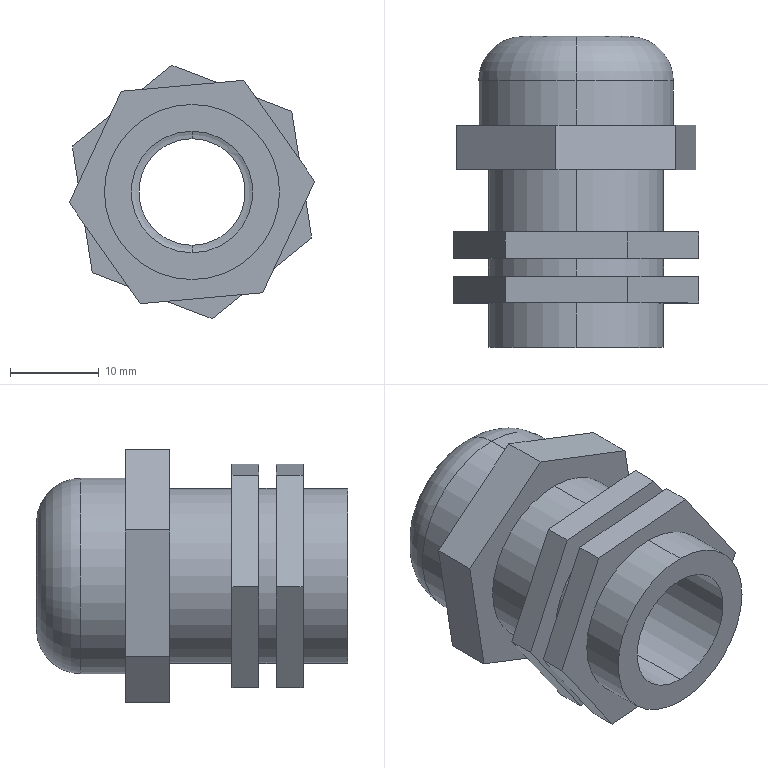Part | SolidWorks | features ICE 5, Extrusion 1, Fillet 1, Shell 1 | 1 solid | 44 faces | box 27.604 x 35 x 28.514 mm | volume 7936 mm3 | plane 26 | cylinder 14 | torus 4 | commonest cylinder face diameters 19.7 x6 12 x2 13.7 x2 16 x2 22 x2
STEP:
#1=CARTESIAN_POINT('',(0.,23.,-6.85));
#2=VERTEX_POINT('',#1);
#3=CARTESIAN_POINT('',(0.,23.,6.85));
#4=VERTEX_POINT('',#3);
#5=CARTESIAN_POINT('',(0.,23.,0.));
#6=DIRECTION('',(0.,1.,0.));
#7=DIRECTION('',(0.,0.,1.));
#8=AXIS2_PLACEMENT_3D('',#5,#6,#7);
#9=CIRCLE('',#8,6.85);
#10=EDGE_CURVE('',#2,#4,#9,.T.);
#11=ORIENTED_EDGE('',*,*,#10,.T.);
#12=CARTESIAN_POINT('',(0.,0.,6.85));
#13=VERTEX_POINT('',#12);
#14=CARTESIAN_POINT('',(0.,20.,6.85));
#15=DIRECTION('',(0.,-1.,0.));
#16=VECTOR('',#15,1000.);
#17=LINE('',#14,#16);
#18=EDGE_CURVE('',#4,#13,#17,.T.);
#19=ORIENTED_EDGE('',*,*,#18,.T.);
#20=CARTESIAN_POINT('',(0.,0.,-6.85));
#21=VERTEX_POINT('',#20);
#22=CARTESIAN_POINT('',(0.,0.,0.));
#23=DIRECTION('',(0.,1.,0.));
#24=DIRECTION('',(0.,0.,1.));
#25=AXIS2_PLACEMENT_3D('',#22,#23,#24);
#26=CIRCLE('',#25,6.85);
#27=EDGE_CURVE('',#21,#13,#26,.T.);
#28=ORIENTED_EDGE('',*,*,#27,.F.);
#29=CARTESIAN_POINT('',(0.,20.,-6.85));
#30=DIRECTION('',(0.,-1.,0.));
#31=VECTOR('',#30,1000.);
#32=LINE('',#29,#31);
#33=EDGE_CURVE('',#2,#21,#32,.T.);
#34=ORIENTED_EDGE('',*,*,#33,.F.);
#35=EDGE_LOOP('',(#11,#19,#28,#34));
#36=FACE_OUTER_BOUND('',#35,.T.);
#37=CARTESIAN_POINT('',(0.,20.,0.));
#38=DIRECTION('',(0.,-1.,0.));
#39=DIRECTION('',(0.,0.,-1.));
#40=AXIS2_PLACEMENT_3D('',#37,#38,#39);
#41=CYLINDRICAL_SURFACE('',#40,6.85);
#42=ADVANCED_FACE('',(#36),#41,.F.);
#43=CARTESIAN_POINT('',(0.,5.,-9.85));
#44=VERTEX_POINT('',#43);
#45=CARTESIAN_POINT('',(0.,5.,9.85));
#46=VERTEX_POINT('',#45);
#47=CARTESIAN_POINT('',(0.,5.,0.));
#48=DIRECTION('',(0.,-1.,0.));
#49=DIRECTION('',(0.,0.,-1.));
#50=AXIS2_PLACEMENT_3D('',#47,#48,#49);
#51=CIRCLE('',#50,9.85);
#52=EDGE_CURVE('',#44,#46,#51,.T.);
#53=ORIENTED_EDGE('',*,*,#52,.T.);
#54=CARTESIAN_POINT('',(0.,0.,9.85));
#55=VERTEX_POINT('',#54);
#56=CARTESIAN_POINT('',(0.,20.,9.85));
#57=DIRECTION('',(0.,-1.,0.));
#58=VECTOR('',#57,1000.);
#59=LINE('',#56,#58);
#60=EDGE_CURVE('',#46,#55,#59,.T.);
#61=ORIENTED_EDGE('',*,*,#60,.T.);
#62=CARTESIAN_POINT('',(0.,0.,-9.85));
#63=VERTEX_POINT('',#62);
#64=CARTESIAN_POINT('',(0.,0.,0.));
#65=DIRECTION('',(0.,1.,0.));
#66=DIRECTION('',(0.,0.,1.));
#67=AXIS2_PLACEMENT_3D('',#64,#65,#66);
#68=CIRCLE('',#67,9.85);
#69=EDGE_CURVE('',#55,#63,#68,.T.);
#70=ORIENTED_EDGE('',*,*,#69,.T.);
#71=CARTESIAN_POINT('',(0.,20.,-9.85));
#72=DIRECTION('',(0.,-1.,0.));
#73=VECTOR('',#72,1000.);
#74=LINE('',#71,#73);
#75=EDGE_CURVE('',#44,#63,#74,.T.);
#76=ORIENTED_EDGE('',*,*,#75,.F.);
#77=EDGE_LOOP('',(#53,#61,#70,#76));
#78=FACE_OUTER_BOUND('',#77,.T.);
#79=CARTESIAN_POINT('',(0.,20.,0.));
#80=DIRECTION('',(0.,-1.,0.));
#81=DIRECTION('',(0.,0.,-1.));
#82=AXIS2_PLACEMENT_3D('',#79,#80,#81);
#83=CYLINDRICAL_SURFACE('',#82,9.85);
#84=ADVANCED_FACE('',(#78),#83,.T.);
#85=CARTESIAN_POINT('',(0.,30.,8.));
#86=VERTEX_POINT('',#85);
#87=CARTESIAN_POINT('',(0.,30.,-8.));
#88=VERTEX_POINT('',#87);
#89=CARTESIAN_POINT('',(0.,30.,0.));
#90=DIRECTION('',(0.,-1.,0.));
#91=DIRECTION('',(0.,0.,-1.));
#92=AXIS2_PLACEMENT_3D('',#89,#90,#91);
#93=CIRCLE('',#92,8.);
#94=EDGE_CURVE('',#86,#88,#93,.T.);
#95=ORIENTED_EDGE('',*,*,#94,.T.);
#96=CARTESIAN_POINT('',(0.,32.,-6.));
#97=VERTEX_POINT('',#96);
#98=CARTESIAN_POINT('',(0.,30.,-6.));
#99=DIRECTION('',(1.,0.,0.));
#100=DIRECTION('',(0.,0.,-1.));
#101=AXIS2_PLACEMENT_3D('',#98,#99,#100);
#102=CIRCLE('',#101,2.);
#103=EDGE_CURVE('',#88,#97,#102,.T.);
#104=ORIENTED_EDGE('',*,*,#103,.T.);
#105=CARTESIAN_POINT('',(0.,32.,6.));
#106=VERTEX_POINT('',#105);
#107=CARTESIAN_POINT('',(0.,32.,0.));
#108=DIRECTION('',(0.,1.,0.));
#109=DIRECTION('',(0.,0.,-1.));
#110=AXIS2_PLACEMENT_3D('',#107,#108,#109);
#111=CIRCLE('',#110,6.);
#112=EDGE_CURVE('',#97,#106,#111,.T.);
#113=ORIENTED_EDGE('',*,*,#112,.T.);
#114=CARTESIAN_POINT('',(0.,30.,6.));
#115=DIRECTION('',(-1.,0.,0.));
#116=DIRECTION('',(0.,0.,1.));
#117=AXIS2_PLACEMENT_3D('',#114,#115,#116);
#118=CIRCLE('',#117,2.);
#119=EDGE_CURVE('',#86,#106,#118,.T.);
#120=ORIENTED_EDGE('',*,*,#119,.F.);
#121=EDGE_LOOP('',(#95,#104,#113,#120));
#122=FACE_OUTER_BOUND('',#121,.T.);
#123=CARTESIAN_POINT('',(0.,30.,0.));
#124=DIRECTION('',(0.,1.,0.));
#125=DIRECTION('',(0.,0.,1.));
#126=AXIS2_PLACEMENT_3D('',#123,#124,#125);
#127=TOROIDAL_SURFACE('',#126,6.,2.);
#128=ADVANCED_FACE('',(#122),#127,.F.);
#129=ORIENTED_EDGE('',*,*,#94,.F.);
#130=CARTESIAN_POINT('',(0.,23.,8.));
#131=VERTEX_POINT('',#130);
#132=CARTESIAN_POINT('',(0.,35.,8.));
#133=DIRECTION('',(0.,-1.,0.));
#134=VECTOR('',#133,1000.);
#135=LINE('',#132,#134);
#136=EDGE_CURVE('',#86,#131,#135,.T.);
#137=ORIENTED_EDGE('',*,*,#136,.T.);
#138=CARTESIAN_POINT('',(0.,23.,-8.));
#139=VERTEX_POINT('',#138);
#140=CARTESIAN_POINT('',(0.,23.,0.));
#141=DIRECTION('',(0.,-1.,0.));
#142=DIRECTION('',(0.,0.,1.));
#143=AXIS2_PLACEMENT_3D('',#140,#141,#142);
#144=CIRCLE('',#143,8.);
#145=EDGE_CURVE('',#131,#139,#144,.T.);
#146=ORIENTED_EDGE('',*,*,#145,.T.);
#147=CARTESIAN_POINT('',(0.,35.,-8.));
#148=DIRECTION('',(0.,-1.,0.));
#149=VECTOR('',#148,1000.);
#150=LINE('',#147,#149);
#151=EDGE_CURVE('',#88,#139,#150,.T.);
#152=ORIENTED_EDGE('',*,*,#151,.F.);
#153=EDGE_LOOP('',(#129,#137,#146,#152));
#154=FACE_OUTER_BOUND('',#153,.T.);
#155=CARTESIAN_POINT('',(0.,35.,0.));
#156=DIRECTION('',(0.,-1.,0.));
#157=DIRECTION('',(0.,0.,-1.));
#158=AXIS2_PLACEMENT_3D('',#155,#156,#157);
#159=CYLINDRICAL_SURFACE('',#158,8.);
#160=ADVANCED_FACE('',(#154),#159,.F.);
#161=ORIENTED_EDGE('',*,*,#112,.F.);
#162=CARTESIAN_POINT('',(0.,35.,-6.));
#163=VERTEX_POINT('',#162);
#164=CARTESIAN_POINT('',(0.,35.,-6.));
#165=DIRECTION('',(0.,1.,0.));
#166=VECTOR('',#165,1000.);
#167=LINE('',#164,#166);
#168=EDGE_CURVE('',#97,#163,#167,.T.);
#169=ORIENTED_EDGE('',*,*,#168,.T.);
#170=CARTESIAN_POINT('',(0.,35.,6.));
#171=VERTEX_POINT('',#170);
#172=CARTESIAN_POINT('',(0.,35.,0.));
#173=DIRECTION('',(0.,1.,0.));
#174=DIRECTION('',(0.,0.,1.));
#175=AXIS2_PLACEMENT_3D('',#172,#173,#174);
#176=CIRCLE('',#175,6.);
#177=EDGE_CURVE('',#163,#171,#176,.T.);
#178=ORIENTED_EDGE('',*,*,#177,.T.);
#179=CARTESIAN_POINT('',(0.,35.,6.));
#180=DIRECTION('',(0.,1.,0.));
#181=VECTOR('',#180,1000.);
#182=LINE('',#179,#181);
#183=EDGE_CURVE('',#106,#171,#182,.T.);
#184=ORIENTED_EDGE('',*,*,#183,.F.);
#185=EDGE_LOOP('',(#161,#169,#178,#184));
#186=FACE_OUTER_BOUND('',#185,.T.);
#187=CARTESIAN_POINT('',(0.,35.,0.));
#188=DIRECTION('',(0.,1.,0.));
#189=DIRECTION('',(0.,0.,1.));
#190=AXIS2_PLACEMENT_3D('',#187,#188,#189);
#191=CYLINDRICAL_SURFACE('',#190,6.);
#192=ADVANCED_FACE('',(#186),#191,.F.);
#193=CARTESIAN_POINT('',(0.,30.,-11.));
#194=VERTEX_POINT('',#193);
#195=CARTESIAN_POINT('',(0.,30.,11.));
#196=VERTEX_POINT('',#195);
#197=CARTESIAN_POINT('',(0.,30.,0.));
#198=DIRECTION('',(0.,-1.,0.));
#199=DIRECTION('',(0.,0.,1.));
#200=AXIS2_PLACEMENT_3D('',#197,#198,#199);
#201=CIRCLE('',#200,11.);
#202=EDGE_CURVE('',#194,#196,#201,.T.);
#203=ORIENTED_EDGE('',*,*,#202,.F.);
#204=CARTESIAN_POINT('',(0.,30.,-6.));
#205=DIRECTION('',(1.,0.,0.));
#206=DIRECTION('',(0.,0.,-1.));
#207=AXIS2_PLACEMENT_3D('',#204,#205,#206);
#208=CIRCLE('',#207,5.);
#209=EDGE_CURVE('',#194,#163,#208,.T.);
#210=ORIENTED_EDGE('',*,*,#209,.T.);
#211=CARTESIAN_POINT('',(0.,35.,0.));
#212=DIRECTION('',(0.,1.,0.));
#213=DIRECTION('',(0.,0.,1.));
#214=AXIS2_PLACEMENT_3D('',#211,#212,#213);
#215=CIRCLE('',#214,6.);
#216=EDGE_CURVE('',#171,#163,#215,.T.);
#217=ORIENTED_EDGE('',*,*,#216,.F.);
#218=CARTESIAN_POINT('',(0.,30.,6.));
#219=DIRECTION('',(-1.,0.,0.));
#220=DIRECTION('',(0.,0.,1.));
#221=AXIS2_PLACEMENT_3D('',#218,#219,#220);
#222=CIRCLE('',#221,5.);
#223=EDGE_CURVE('',#196,#171,#222,.T.);
#224=ORIENTED_EDGE('',*,*,#223,.F.);
#225=EDGE_LOOP('',(#203,#210,#217,#224));
#226=FACE_OUTER_BOUND('',#225,.T.);
#227=CARTESIAN_POINT('',(0.,30.,0.));
#228=DIRECTION('',(0.,1.,0.));
#229=DIRECTION('',(0.,0.,1.));
#230=AXIS2_PLACEMENT_3D('',#227,#228,#229);
#231=TOROIDAL_SURFACE('',#230,6.,5.);
#232=ADVANCED_FACE('',(#226),#231,.T.);
#233=ORIENTED_EDGE('',*,*,#202,.T.);
#234=CARTESIAN_POINT('',(0.,25.,11.));
#235=VERTEX_POINT('',#234);
#236=CARTESIAN_POINT('',(0.,35.,11.));
#237=DIRECTION('',(0.,-1.,0.));
#238=VECTOR('',#237,1000.);
#239=LINE('',#236,#238);
#240=EDGE_CURVE('',#196,#235,#239,.T.);
#241=ORIENTED_EDGE('',*,*,#240,.T.);
#242=CARTESIAN_POINT('',(0.,25.,-11.));
#243=VERTEX_POINT('',#242);
#244=CARTESIAN_POINT('',(0.,25.,0.));
#245=DIRECTION('',(0.,1.,0.));
#246=DIRECTION('',(0.,0.,1.));
#247=AXIS2_PLACEMENT_3D('',#244,#245,#246);
#248=CIRCLE('',#247,11.);
#249=EDGE_CURVE('',#235,#243,#248,.T.);
#250=ORIENTED_EDGE('',*,*,#249,.T.);
#251=CARTESIAN_POINT('',(0.,35.,-11.));
#252=DIRECTION('',(0.,-1.,0.));
#253=VECTOR('',#252,1000.);
#254=LINE('',#251,#253);
#255=EDGE_CURVE('',#194,#243,#254,.T.);
#256=ORIENTED_EDGE('',*,*,#255,.F.);
#257=EDGE_LOOP('',(#233,#241,#250,#256));
#258=FACE_OUTER_BOUND('',#257,.T.);
#259=CARTESIAN_POINT('',(0.,35.,0.));
#260=DIRECTION('',(0.,-1.,0.));
#261=DIRECTION('',(0.,0.,-1.));
#262=AXIS2_PLACEMENT_3D('',#259,#260,#261);
#263=CYLINDRICAL_SURFACE('',#262,11.);
#264=ADVANCED_FACE('',(#258),#263,.T.);
#265=CARTESIAN_POINT('',(0.,20.,9.85));
#266=VERTEX_POINT('',#265);
#267=CARTESIAN_POINT('',(0.,20.,-9.85));
#268=VERTEX_POINT('',#267);
#269=CARTESIAN_POINT('',(0.,20.,0.));
#270=DIRECTION('',(0.,1.,0.));
#271=DIRECTION('',(0.,0.,1.));
#272=AXIS2_PLACEMENT_3D('',#269,#270,#271);
#273=CIRCLE('',#272,9.85);
#274=EDGE_CURVE('',#266,#268,#273,.T.);
#275=ORIENTED_EDGE('',*,*,#274,.F.);
#276=CARTESIAN_POINT('',(0.,13.,9.85));
#277=VERTEX_POINT('',#276);
#278=CARTESIAN_POINT('',(0.,20.,9.85));
#279=DIRECTION('',(0.,-1.,0.));
#280=VECTOR('',#279,1000.);
#281=LINE('',#278,#280);
#282=EDGE_CURVE('',#266,#277,#281,.T.);
#283=ORIENTED_EDGE('',*,*,#282,.T.);
#284=CARTESIAN_POINT('',(0.,13.,-9.85));
#285=VERTEX_POINT('',#284);
#286=CARTESIAN_POINT('',(0.,13.,0.));
#287=DIRECTION('',(0.,-1.,0.));
#288=DIRECTION('',(0.,0.,-1.));
#289=AXIS2_PLACEMENT_3D('',#286,#287,#288);
#290=CIRCLE('',#289,9.85);
#291=EDGE_CURVE('',#285,#277,#290,.T.);
#292=ORIENTED_EDGE('',*,*,#291,.F.);
#293=CARTESIAN_POINT('',(0.,20.,-9.85));
#294=DIRECTION('',(0.,-1.,0.));
#295=VECTOR('',#294,1000.);
#296=LINE('',#293,#295);
#297=EDGE_CURVE('',#268,#285,#296,.T.);
#298=ORIENTED_EDGE('',*,*,#297,.F.);
#299=EDGE_LOOP('',(#275,#283,#292,#298));
#300=FACE_OUTER_BOUND('',#299,.T.);
#301=CARTESIAN_POINT('',(0.,20.,0.));
#302=DIRECTION('',(0.,-1.,0.));
#303=DIRECTION('',(0.,0.,-1.));
#304=AXIS2_PLACEMENT_3D('',#301,#302,#303);
#305=CYLINDRICAL_SURFACE('',#304,9.85);
#306=ADVANCED_FACE('',(#300),#305,.T.);
#307=CARTESIAN_POINT('',(0.,10.,-9.85));
#308=VERTEX_POINT('',#307);
#309=CARTESIAN_POINT('',(0.,10.,9.85));
#310=VERTEX_POINT('',#309);
#311=CARTESIAN_POINT('',(0.,10.,0.));
#312=DIRECTION('',(0.,-1.,0.));
#313=DIRECTION('',(0.,0.,-1.));
#314=AXIS2_PLACEMENT_3D('',#311,#312,#313);
#315=CIRCLE('',#314,9.85);
#316=EDGE_CURVE('',#308,#310,#315,.T.);
#317=ORIENTED_EDGE('',*,*,#316,.T.);
#318=CARTESIAN_POINT('',(0.,8.,9.85));
#319=VERTEX_POINT('',#318);
#320=CARTESIAN_POINT('',(0.,20.,9.85));
#321=DIRECTION('',(0.,-1.,0.));
#322=VECTOR('',#321,1000.);
#323=LINE('',#320,#322);
#324=EDGE_CURVE('',#310,#319,#323,.T.);
#325=ORIENTED_EDGE('',*,*,#324,.T.);
#326=CARTESIAN_POINT('',(0.,8.,-9.85));
#327=VERTEX_POINT('',#326);
#328=CARTESIAN_POINT('',(0.,8.,0.));
#329=DIRECTION('',(0.,-1.,0.));
#330=DIRECTION('',(0.,0.,-1.));
#331=AXIS2_PLACEMENT_3D('',#328,#329,#330);
#332=CIRCLE('',#331,9.85);
#333=EDGE_CURVE('',#327,#319,#332,.T.);
#334=ORIENTED_EDGE('',*,*,#333,.F.);
#335=CARTESIAN_POINT('',(0.,20.,-9.85));
#336=DIRECTION('',(0.,-1.,0.));
#337=VECTOR('',#336,1000.);
#338=LINE('',#335,#337);
#339=EDGE_CURVE('',#308,#327,#338,.T.);
#340=ORIENTED_EDGE('',*,*,#339,.F.);
#341=EDGE_LOOP('',(#317,#325,#334,#340));
#342=FACE_OUTER_BOUND('',#341,.T.);
#343=CARTESIAN_POINT('',(0.,20.,0.));
#344=DIRECTION('',(0.,-1.,0.));
#345=DIRECTION('',(0.,0.,-1.));
#346=AXIS2_PLACEMENT_3D('',#343,#344,#345);
#347=CYLINDRICAL_SURFACE('',#346,9.85);
#348=ADVANCED_FACE('',(#342),#347,.T.);
#349=ORIENTED_EDGE('',*,*,#324,.F.);
#350=CARTESIAN_POINT('',(0.,10.,0.));
#351=DIRECTION('',(0.,-1.,0.));
#352=DIRECTION('',(0.,0.,-1.));
#353=AXIS2_PLACEMENT_3D('',#350,#351,#352);
#354=CIRCLE('',#353,9.85);
#355=EDGE_CURVE('',#310,#308,#354,.T.);
#356=ORIENTED_EDGE('',*,*,#355,.T.);
#357=ORIENTED_EDGE('',*,*,#339,.T.);
#358=CARTESIAN_POINT('',(0.,8.,0.));
#359=DIRECTION('',(0.,-1.,0.));
#360=DIRECTION('',(0.,0.,-1.));
#361=AXIS2_PLACEMENT_3D('',#358,#359,#360);
#362=CIRCLE('',#361,9.85);
#363=EDGE_CURVE('',#319,#327,#362,.T.);
#364=ORIENTED_EDGE('',*,*,#363,.F.);
#365=EDGE_LOOP('',(#349,#356,#357,#364));
#366=FACE_OUTER_BOUND('',#365,.T.);
#367=CARTESIAN_POINT('',(0.,20.,0.));
#368=DIRECTION('',(0.,-1.,0.));
#369=DIRECTION('',(0.,0.,-1.));
#370=AXIS2_PLACEMENT_3D('',#367,#368,#369);
#371=CYLINDRICAL_SURFACE('',#370,9.85);
#372=ADVANCED_FACE('',(#366),#371,.T.);
#373=ORIENTED_EDGE('',*,*,#282,.F.);
#374=CARTESIAN_POINT('',(0.,20.,0.));
#375=DIRECTION('',(0.,1.,0.));
#376=DIRECTION('',(0.,0.,1.));
#377=AXIS2_PLACEMENT_3D('',#374,#375,#376);
#378=CIRCLE('',#377,9.85);
#379=EDGE_CURVE('',#268,#266,#378,.T.);
#380=ORIENTED_EDGE('',*,*,#379,.F.);
#381=ORIENTED_EDGE('',*,*,#297,.T.);
#382=CARTESIAN_POINT('',(0.,13.,0.));
#383=DIRECTION('',(0.,-1.,0.));
#384=DIRECTION('',(0.,0.,-1.));
#385=AXIS2_PLACEMENT_3D('',#382,#383,#384);
#386=CIRCLE('',#385,9.85);
#387=EDGE_CURVE('',#277,#285,#386,.T.);
#388=ORIENTED_EDGE('',*,*,#387,.F.);
#389=EDGE_LOOP('',(#373,#380,#381,#388));
#390=FACE_OUTER_BOUND('',#389,.T.);
#391=CARTESIAN_POINT('',(0.,20.,0.));
#392=DIRECTION('',(0.,-1.,0.));
#393=DIRECTION('',(0.,0.,-1.));
#394=AXIS2_PLACEMENT_3D('',#391,#392,#393);
#395=CYLINDRICAL_SURFACE('',#394,9.85);
#396=ADVANCED_FACE('',(#390),#395,.T.);
#397=CARTESIAN_POINT('',(13.473,20.,-5.178));
#398=VERTEX_POINT('',#397);
#399=CARTESIAN_POINT('',(2.253,20.,-14.257));
#400=VERTEX_POINT('',#399);
#401=CARTESIAN_POINT('',(13.473,20.,-5.178));
#402=DIRECTION('',(-0.7774,0.,-0.629));
#403=VECTOR('',#402,1000.);
#404=LINE('',#401,#403);
#405=EDGE_CURVE('',#398,#400,#404,.T.);
#406=ORIENTED_EDGE('',*,*,#405,.T.);
#407=CARTESIAN_POINT('',(2.253,25.,-14.257));
#408=VERTEX_POINT('',#407);
#409=CARTESIAN_POINT('',(2.253,25.,-14.257));
#410=DIRECTION('',(0.,-1.,0.));
#411=VECTOR('',#410,1000.);
#412=LINE('',#409,#411);
#413=EDGE_CURVE('',#408,#400,#412,.T.);
#414=ORIENTED_EDGE('',*,*,#413,.F.);
#415=CARTESIAN_POINT('',(13.473,25.,-5.178));
#416=VERTEX_POINT('',#415);
#417=CARTESIAN_POINT('',(13.473,25.,-5.178));
#418=DIRECTION('',(-0.7774,0.,-0.629));
#419=VECTOR('',#418,1000.);
#420=LINE('',#417,#419);
#421=EDGE_CURVE('',#416,#408,#420,.T.);
#422=ORIENTED_EDGE('',*,*,#421,.F.);
#423=CARTESIAN_POINT('',(13.473,25.,-5.178));
#424=DIRECTION('',(0.,-1.,0.));
#425=VECTOR('',#424,1000.);
#426=LINE('',#423,#425);
#427=EDGE_CURVE('',#416,#398,#426,.T.);
#428=ORIENTED_EDGE('',*,*,#427,.T.);
#429=EDGE_LOOP('',(#406,#414,#422,#428));
#430=FACE_OUTER_BOUND('',#429,.T.);
#431=CARTESIAN_POINT('',(13.473,25.,-5.178));
#432=DIRECTION('',(-0.629,0.,0.7774));
#433=DIRECTION('',(0.7774,0.,0.629));
#434=AXIS2_PLACEMENT_3D('',#431,#432,#433);
#435=PLANE('',#434);
#436=ADVANCED_FACE('',(#430),#435,.F.);
#437=CARTESIAN_POINT('',(-11.221,20.,-9.079));
#438=VERTEX_POINT('',#437);
#439=CARTESIAN_POINT('',(2.253,20.,-14.257));
#440=DIRECTION('',(-0.9334,0.,0.3587));
#441=VECTOR('',#440,1000.);
#442=LINE('',#439,#441);
#443=EDGE_CURVE('',#400,#438,#442,.T.);
#444=ORIENTED_EDGE('',*,*,#443,.T.);
#445=CARTESIAN_POINT('',(-11.221,25.,-9.079));
#446=VERTEX_POINT('',#445);
#447=CARTESIAN_POINT('',(-11.221,25.,-9.079));
#448=DIRECTION('',(0.,-1.,0.));
#449=VECTOR('',#448,1000.);
#450=LINE('',#447,#449);
#451=EDGE_CURVE('',#446,#438,#450,.T.);
#452=ORIENTED_EDGE('',*,*,#451,.F.);
#453=CARTESIAN_POINT('',(2.253,25.,-14.257));
#454=DIRECTION('',(-0.9334,0.,0.3587));
#455=VECTOR('',#454,1000.);
#456=LINE('',#453,#455);
#457=EDGE_CURVE('',#408,#446,#456,.T.);
#458=ORIENTED_EDGE('',*,*,#457,.F.);
#459=ORIENTED_EDGE('',*,*,#413,.T.);
#460=EDGE_LOOP('',(#444,#452,#458,#459));
#461=FACE_OUTER_BOUND('',#460,.T.);
#462=CARTESIAN_POINT('',(2.253,25.,-14.257));
#463=DIRECTION('',(0.3587,0.,0.9334));
#464=DIRECTION('',(0.9334,0.,-0.3587));
#465=AXIS2_PLACEMENT_3D('',#462,#463,#464);
#466=PLANE('',#465);
#467=ADVANCED_FACE('',(#461),#466,.F.);
#468=CARTESIAN_POINT('',(-13.473,20.,5.178));
#469=VERTEX_POINT('',#468);
#470=CARTESIAN_POINT('',(-11.221,20.,-9.079));
#471=DIRECTION('',(-0.1561,0.,0.9877));
#472=VECTOR('',#471,1000.);
#473=LINE('',#470,#472);
#474=EDGE_CURVE('',#438,#469,#473,.T.);
#475=ORIENTED_EDGE('',*,*,#474,.T.);
#476=CARTESIAN_POINT('',(-13.473,25.,5.178));
#477=VERTEX_POINT('',#476);
#478=CARTESIAN_POINT('',(-13.473,25.,5.178));
#479=DIRECTION('',(0.,-1.,0.));
#480=VECTOR('',#479,1000.);
#481=LINE('',#478,#480);
#482=EDGE_CURVE('',#477,#469,#481,.T.);
#483=ORIENTED_EDGE('',*,*,#482,.F.);
#484=CARTESIAN_POINT('',(-11.221,25.,-9.079));
#485=DIRECTION('',(-0.1561,0.,0.9877));
#486=VECTOR('',#485,1000.);
#487=LINE('',#484,#486);
#488=EDGE_CURVE('',#446,#477,#487,.T.);
#489=ORIENTED_EDGE('',*,*,#488,.F.);
#490=ORIENTED_EDGE('',*,*,#451,.T.);
#491=EDGE_LOOP('',(#475,#483,#489,#490));
#492=FACE_OUTER_BOUND('',#491,.T.);
#493=CARTESIAN_POINT('',(-11.221,25.,-9.079));
#494=DIRECTION('',(0.9877,0.,0.1561));
#495=DIRECTION('',(0.1561,0.,-0.9877));
#496=AXIS2_PLACEMENT_3D('',#493,#494,#495);
#497=PLANE('',#496);
#498=ADVANCED_FACE('',(#492),#497,.F.);
#499=CARTESIAN_POINT('',(-2.253,20.,14.257));
#500=VERTEX_POINT('',#499);
#501=CARTESIAN_POINT('',(-13.473,20.,5.178));
#502=DIRECTION('',(0.7774,0.,0.629));
#503=VECTOR('',#502,1000.);
#504=LINE('',#501,#503);
#505=EDGE_CURVE('',#469,#500,#504,.T.);
#506=ORIENTED_EDGE('',*,*,#505,.T.);
#507=CARTESIAN_POINT('',(-2.253,25.,14.257));
#508=VERTEX_POINT('',#507);
#509=CARTESIAN_POINT('',(-2.253,25.,14.257));
#510=DIRECTION('',(0.,-1.,0.));
#511=VECTOR('',#510,1000.);
#512=LINE('',#509,#511);
#513=EDGE_CURVE('',#508,#500,#512,.T.);
#514=ORIENTED_EDGE('',*,*,#513,.F.);
#515=CARTESIAN_POINT('',(-13.473,25.,5.178));
#516=DIRECTION('',(0.7774,0.,0.629));
#517=VECTOR('',#516,1000.);
#518=LINE('',#515,#517);
#519=EDGE_CURVE('',#477,#508,#518,.T.);
#520=ORIENTED_EDGE('',*,*,#519,.F.);
#521=ORIENTED_EDGE('',*,*,#482,.T.);
#522=EDGE_LOOP('',(#506,#514,#520,#521));
#523=FACE_OUTER_BOUND('',#522,.T.);
#524=CARTESIAN_POINT('',(-13.473,25.,5.178));
#525=DIRECTION('',(0.629,0.,-0.7774));
#526=DIRECTION('',(-0.7774,0.,-0.629));
#527=AXIS2_PLACEMENT_3D('',#524,#525,#526);
#528=PLANE('',#527);
#529=ADVANCED_FACE('',(#523),#528,.F.);
#530=CARTESIAN_POINT('',(11.221,20.,9.079));
#531=VERTEX_POINT('',#530);
#532=CARTESIAN_POINT('',(-2.253,20.,14.257));
#533=DIRECTION('',(0.9334,0.,-0.3587));
#534=VECTOR('',#533,1000.);
#535=LINE('',#532,#534);
#536=EDGE_CURVE('',#500,#531,#535,.T.);
#537=ORIENTED_EDGE('',*,*,#536,.T.);
#538=CARTESIAN_POINT('',(11.221,25.,9.079));
#539=VERTEX_POINT('',#538);
#540=CARTESIAN_POINT('',(11.221,25.,9.079));
#541=DIRECTION('',(0.,-1.,0.));
#542=VECTOR('',#541,1000.);
#543=LINE('',#540,#542);
#544=EDGE_CURVE('',#539,#531,#543,.T.);
#545=ORIENTED_EDGE('',*,*,#544,.F.);
#546=CARTESIAN_POINT('',(-2.253,25.,14.257));
#547=DIRECTION('',(0.9334,0.,-0.3587));
#548=VECTOR('',#547,1000.);
#549=LINE('',#546,#548);
#550=EDGE_CURVE('',#508,#539,#549,.T.);
#551=ORIENTED_EDGE('',*,*,#550,.F.);
#552=ORIENTED_EDGE('',*,*,#513,.T.);
#553=EDGE_LOOP('',(#537,#545,#551,#552));
#554=FACE_OUTER_BOUND('',#553,.T.);
#555=CARTESIAN_POINT('',(-2.253,25.,14.257));
#556=DIRECTION('',(-0.3587,0.,-0.9334));
#557=DIRECTION('',(-0.9334,0.,0.3587));
#558=AXIS2_PLACEMENT_3D('',#555,#556,#557);
#559=PLANE('',#558);
#560=ADVANCED_FACE('',(#554),#559,.F.);
#561=CARTESIAN_POINT('',(11.221,20.,9.079));
#562=DIRECTION('',(0.1561,0.,-0.9877));
#563=VECTOR('',#562,1000.);
#564=LINE('',#561,#563);
#565=EDGE_CURVE('',#531,#398,#564,.T.);
#566=ORIENTED_EDGE('',*,*,#565,.T.);
#567=ORIENTED_EDGE('',*,*,#427,.F.);
#568=CARTESIAN_POINT('',(11.221,25.,9.079));
#569=DIRECTION('',(0.1561,0.,-0.9877));
#570=VECTOR('',#569,1000.);
#571=LINE('',#568,#570);
#572=EDGE_CURVE('',#539,#416,#571,.T.);
#573=ORIENTED_EDGE('',*,*,#572,.F.);
#574=ORIENTED_EDGE('',*,*,#544,.T.);
#575=EDGE_LOOP('',(#566,#567,#573,#574));
#576=FACE_OUTER_BOUND('',#575,.T.);
#577=CARTESIAN_POINT('',(11.221,25.,9.079));
#578=DIRECTION('',(-0.9877,0.,-0.1561));
#579=DIRECTION('',(-0.1561,0.,0.9877));
#580=AXIS2_PLACEMENT_3D('',#577,#578,#579);
#581=PLANE('',#580);
#582=ADVANCED_FACE('',(#576),#581,.F.);
#583=CARTESIAN_POINT('',(0.,25.,0.));
#584=DIRECTION('',(0.,1.,0.));
#585=DIRECTION('',(0.,0.,1.));
#586=AXIS2_PLACEMENT_3D('',#583,#584,#585);
#587=CIRCLE('',#586,11.);
#588=EDGE_CURVE('',#243,#235,#587,.T.);
#589=ORIENTED_EDGE('',*,*,#588,.F.);
#590=ORIENTED_EDGE('',*,*,#249,.F.);
#591=EDGE_LOOP('',(#589,#590));
#592=FACE_BOUND('',#591,.T.);
#593=ORIENTED_EDGE('',*,*,#421,.T.);
#594=ORIENTED_EDGE('',*,*,#457,.T.);
#595=ORIENTED_EDGE('',*,*,#488,.T.);
#596=ORIENTED_EDGE('',*,*,#519,.T.);
#597=ORIENTED_EDGE('',*,*,#550,.T.);
#598=ORIENTED_EDGE('',*,*,#572,.T.);
#599=EDGE_LOOP('',(#593,#594,#595,#596,#597,#598));
#600=FACE_OUTER_BOUND('',#599,.T.);
#601=CARTESIAN_POINT('',(0.,25.,0.));
#602=DIRECTION('',(0.,1.,0.));
#603=DIRECTION('',(0.,0.,1.));
#604=AXIS2_PLACEMENT_3D('',#601,#602,#603);
#605=PLANE('',#604);
#606=ADVANCED_FACE('',(#592,#600),#605,.T.);
#607=ORIENTED_EDGE('',*,*,#379,.T.);
#608=ORIENTED_EDGE('',*,*,#274,.T.);
#609=EDGE_LOOP('',(#607,#608));
#610=FACE_BOUND('',#609,.T.);
#611=ORIENTED_EDGE('',*,*,#405,.F.);
#612=ORIENTED_EDGE('',*,*,#565,.F.);
#613=ORIENTED_EDGE('',*,*,#536,.F.);
#614=ORIENTED_EDGE('',*,*,#505,.F.);
#615=ORIENTED_EDGE('',*,*,#474,.F.);
#616=ORIENTED_EDGE('',*,*,#443,.F.);
#617=EDGE_LOOP('',(#611,#612,#613,#614,#615,#616));
#618=FACE_OUTER_BOUND('',#617,.T.);
#619=CARTESIAN_POINT('',(0.,20.,0.));
#620=DIRECTION('',(0.,1.,0.));
#621=DIRECTION('',(0.,0.,1.));
#622=AXIS2_PLACEMENT_3D('',#619,#620,#621);
#623=PLANE('',#622);
#624=ADVANCED_FACE('',(#610,#618),#623,.F.);
#625=ORIENTED_EDGE('',*,*,#240,.F.);
#626=CARTESIAN_POINT('',(0.,30.,0.));
#627=DIRECTION('',(0.,-1.,0.));
#628=DIRECTION('',(0.,0.,1.));
#629=AXIS2_PLACEMENT_3D('',#626,#627,#628);
#630=CIRCLE('',#629,11.);
#631=EDGE_CURVE('',#196,#194,#630,.T.);
#632=ORIENTED_EDGE('',*,*,#631,.T.);
#633=ORIENTED_EDGE('',*,*,#255,.T.);
#634=ORIENTED_EDGE('',*,*,#588,.T.);
#635=EDGE_LOOP('',(#625,#632,#633,#634));
#636=FACE_OUTER_BOUND('',#635,.T.);
#637=CARTESIAN_POINT('',(0.,35.,0.));
#638=DIRECTION('',(0.,-1.,0.));
#639=DIRECTION('',(0.,0.,-1.));
#640=AXIS2_PLACEMENT_3D('',#637,#638,#639);
#641=CYLINDRICAL_SURFACE('',#640,11.);
#642=ADVANCED_FACE('',(#636),#641,.T.);
#643=ORIENTED_EDGE('',*,*,#209,.F.);
#644=ORIENTED_EDGE('',*,*,#631,.F.);
#645=ORIENTED_EDGE('',*,*,#223,.T.);
#646=ORIENTED_EDGE('',*,*,#177,.F.);
#647=EDGE_LOOP('',(#643,#644,#645,#646));
#648=FACE_OUTER_BOUND('',#647,.T.);
#649=CARTESIAN_POINT('',(0.,30.,0.));
#650=DIRECTION('',(0.,1.,0.));
#651=DIRECTION('',(0.,0.,1.));
#652=AXIS2_PLACEMENT_3D('',#649,#650,#651);
#653=TOROIDAL_SURFACE('',#652,6.,5.);
#654=ADVANCED_FACE('',(#648),#653,.T.);
#655=ORIENTED_EDGE('',*,*,#10,.F.);
#656=CARTESIAN_POINT('',(0.,23.,0.));
#657=DIRECTION('',(0.,1.,0.));
#658=DIRECTION('',(0.,0.,1.));
#659=AXIS2_PLACEMENT_3D('',#656,#657,#658);
#660=CIRCLE('',#659,6.85);
#661=EDGE_CURVE('',#4,#2,#660,.T.);
#662=ORIENTED_EDGE('',*,*,#661,.F.);
#663=EDGE_LOOP('',(#655,#662));
#664=FACE_BOUND('',#663,.T.);
#665=CARTESIAN_POINT('',(0.,23.,0.));
#666=DIRECTION('',(0.,-1.,0.));
#667=DIRECTION('',(0.,0.,1.));
#668=AXIS2_PLACEMENT_3D('',#665,#666,#667);
#669=CIRCLE('',#668,8.);
#670=EDGE_CURVE('',#139,#131,#669,.T.);
#671=ORIENTED_EDGE('',*,*,#670,.F.);
#672=ORIENTED_EDGE('',*,*,#145,.F.);
#673=EDGE_LOOP('',(#671,#672));
#674=FACE_OUTER_BOUND('',#673,.T.);
#675=CARTESIAN_POINT('',(0.,23.,0.));
#676=DIRECTION('',(0.,1.,0.));
#677=DIRECTION('',(0.,0.,1.));
#678=AXIS2_PLACEMENT_3D('',#675,#676,#677);
#679=PLANE('',#678);
#680=ADVANCED_FACE('',(#664,#674),#679,.T.);
#681=ORIENTED_EDGE('',*,*,#168,.F.);
#682=CARTESIAN_POINT('',(0.,32.,0.));
#683=DIRECTION('',(0.,1.,0.));
#684=DIRECTION('',(0.,0.,-1.));
#685=AXIS2_PLACEMENT_3D('',#682,#683,#684);
#686=CIRCLE('',#685,6.);
#687=EDGE_CURVE('',#106,#97,#686,.T.);
#688=ORIENTED_EDGE('',*,*,#687,.F.);
#689=ORIENTED_EDGE('',*,*,#183,.T.);
#690=ORIENTED_EDGE('',*,*,#216,.T.);
#691=EDGE_LOOP('',(#681,#688,#689,#690));
#692=FACE_OUTER_BOUND('',#691,.T.);
#693=CARTESIAN_POINT('',(0.,35.,0.));
#694=DIRECTION('',(0.,1.,0.));
#695=DIRECTION('',(0.,0.,1.));
#696=AXIS2_PLACEMENT_3D('',#693,#694,#695);
#697=CYLINDRICAL_SURFACE('',#696,6.);
#698=ADVANCED_FACE('',(#692),#697,.F.);
#699=ORIENTED_EDGE('',*,*,#136,.F.);
#700=CARTESIAN_POINT('',(0.,30.,0.));
#701=DIRECTION('',(0.,-1.,0.));
#702=DIRECTION('',(0.,0.,-1.));
#703=AXIS2_PLACEMENT_3D('',#700,#701,#702);
#704=CIRCLE('',#703,8.);
#705=EDGE_CURVE('',#88,#86,#704,.T.);
#706=ORIENTED_EDGE('',*,*,#705,.F.);
#707=ORIENTED_EDGE('',*,*,#151,.T.);
#708=ORIENTED_EDGE('',*,*,#670,.T.);
#709=EDGE_LOOP('',(#699,#706,#707,#708));
#710=FACE_OUTER_BOUND('',#709,.T.);
#711=CARTESIAN_POINT('',(0.,35.,0.));
#712=DIRECTION('',(0.,-1.,0.));
#713=DIRECTION('',(0.,0.,-1.));
#714=AXIS2_PLACEMENT_3D('',#711,#712,#713);
#715=CYLINDRICAL_SURFACE('',#714,8.);
#716=ADVANCED_FACE('',(#710),#715,.F.);
#717=ORIENTED_EDGE('',*,*,#103,.F.);
#718=ORIENTED_EDGE('',*,*,#705,.T.);
#719=ORIENTED_EDGE('',*,*,#119,.T.);
#720=ORIENTED_EDGE('',*,*,#687,.T.);
#721=EDGE_LOOP('',(#717,#718,#719,#720));
#722=FACE_OUTER_BOUND('',#721,.T.);
#723=CARTESIAN_POINT('',(0.,30.,0.));
#724=DIRECTION('',(0.,1.,0.));
#725=DIRECTION('',(0.,0.,1.));
#726=AXIS2_PLACEMENT_3D('',#723,#724,#725);
#727=TOROIDAL_SURFACE('',#726,6.,2.);
#728=ADVANCED_FACE('',(#722),#727,.F.);
#729=CARTESIAN_POINT('',(-13.802,10.,-1.229));
#730=VERTEX_POINT('',#729);
#731=CARTESIAN_POINT('',(-5.837,10.,-12.567));
#732=VERTEX_POINT('',#731);
#733=CARTESIAN_POINT('',(-13.802,10.,-1.229));
#734=DIRECTION('',(0.5748,0.,-0.8183));
#735=VECTOR('',#734,1000.);
#736=LINE('',#733,#735);
#737=EDGE_CURVE('',#730,#732,#736,.T.);
#738=ORIENTED_EDGE('',*,*,#737,.F.);
#739=CARTESIAN_POINT('',(-13.802,13.,-1.229));
#740=VERTEX_POINT('',#739);
#741=CARTESIAN_POINT('',(-13.802,13.,-1.229));
#742=DIRECTION('',(0.,-1.,0.));
#743=VECTOR('',#742,1000.);
#744=LINE('',#741,#743);
#745=EDGE_CURVE('',#740,#730,#744,.T.);
#746=ORIENTED_EDGE('',*,*,#745,.F.);
#747=CARTESIAN_POINT('',(-5.837,13.,-12.567));
#748=VERTEX_POINT('',#747);
#749=CARTESIAN_POINT('',(-13.802,13.,-1.229));
#750=DIRECTION('',(0.5748,0.,-0.8183));
#751=VECTOR('',#750,1000.);
#752=LINE('',#749,#751);
#753=EDGE_CURVE('',#740,#748,#752,.T.);
#754=ORIENTED_EDGE('',*,*,#753,.T.);
#755=CARTESIAN_POINT('',(-5.837,13.,-12.567));
#756=DIRECTION('',(0.,-1.,0.));
#757=VECTOR('',#756,1000.);
#758=LINE('',#755,#757);
#759=EDGE_CURVE('',#748,#732,#758,.T.);
#760=ORIENTED_EDGE('',*,*,#759,.T.);
#761=EDGE_LOOP('',(#738,#746,#754,#760));
#762=FACE_OUTER_BOUND('',#761,.T.);
#763=CARTESIAN_POINT('',(-13.802,13.,-1.229));
#764=DIRECTION('',(-0.8183,0.,-0.5748));
#765=DIRECTION('',(-0.5748,0.,0.8183));
#766=AXIS2_PLACEMENT_3D('',#763,#764,#765);
#767=PLANE('',#766);
#768=ADVANCED_FACE('',(#762),#767,.T.);
#769=CARTESIAN_POINT('',(-7.965,10.,11.338));
#770=VERTEX_POINT('',#769);
#771=CARTESIAN_POINT('',(-7.965,10.,11.338));
#772=DIRECTION('',(-0.4212,0.,-0.907));
#773=VECTOR('',#772,1000.);
#774=LINE('',#771,#773);
#775=EDGE_CURVE('',#770,#730,#774,.T.);
#776=ORIENTED_EDGE('',*,*,#775,.F.);
#777=CARTESIAN_POINT('',(-7.965,13.,11.338));
#778=VERTEX_POINT('',#777);
#779=CARTESIAN_POINT('',(-7.965,13.,11.338));
#780=DIRECTION('',(0.,-1.,0.));
#781=VECTOR('',#780,1000.);
#782=LINE('',#779,#781);
#783=EDGE_CURVE('',#778,#770,#782,.T.);
#784=ORIENTED_EDGE('',*,*,#783,.F.);
#785=CARTESIAN_POINT('',(-7.965,13.,11.338));
#786=DIRECTION('',(-0.4212,0.,-0.907));
#787=VECTOR('',#786,1000.);
#788=LINE('',#785,#787);
#789=EDGE_CURVE('',#778,#740,#788,.T.);
#790=ORIENTED_EDGE('',*,*,#789,.T.);
#791=ORIENTED_EDGE('',*,*,#745,.T.);
#792=EDGE_LOOP('',(#776,#784,#790,#791));
#793=FACE_OUTER_BOUND('',#792,.T.);
#794=CARTESIAN_POINT('',(-7.965,13.,11.338));
#795=DIRECTION('',(-0.907,0.,0.4212));
#796=DIRECTION('',(0.4212,0.,0.907));
#797=AXIS2_PLACEMENT_3D('',#794,#795,#796);
#798=PLANE('',#797);
#799=ADVANCED_FACE('',(#793),#798,.T.);
#800=CARTESIAN_POINT('',(5.837,10.,12.567));
#801=VERTEX_POINT('',#800);
#802=CARTESIAN_POINT('',(5.837,10.,12.567));
#803=DIRECTION('',(-0.9961,0.,-0.08869));
#804=VECTOR('',#803,1000.);
#805=LINE('',#802,#804);
#806=EDGE_CURVE('',#801,#770,#805,.T.);
#807=ORIENTED_EDGE('',*,*,#806,.F.);
#808=CARTESIAN_POINT('',(5.837,13.,12.567));
#809=VERTEX_POINT('',#808);
#810=CARTESIAN_POINT('',(5.837,13.,12.567));
#811=DIRECTION('',(0.,-1.,0.));
#812=VECTOR('',#811,1000.);
#813=LINE('',#810,#812);
#814=EDGE_CURVE('',#809,#801,#813,.T.);
#815=ORIENTED_EDGE('',*,*,#814,.F.);
#816=CARTESIAN_POINT('',(5.837,13.,12.567));
#817=DIRECTION('',(-0.9961,0.,-0.08869));
#818=VECTOR('',#817,1000.);
#819=LINE('',#816,#818);
#820=EDGE_CURVE('',#809,#778,#819,.T.);
#821=ORIENTED_EDGE('',*,*,#820,.T.);
#822=ORIENTED_EDGE('',*,*,#783,.T.);
#823=EDGE_LOOP('',(#807,#815,#821,#822));
#824=FACE_OUTER_BOUND('',#823,.T.);
#825=CARTESIAN_POINT('',(5.837,13.,12.567));
#826=DIRECTION('',(-0.08869,0.,0.9961));
#827=DIRECTION('',(0.9961,0.,0.08869));
#828=AXIS2_PLACEMENT_3D('',#825,#826,#827);
#829=PLANE('',#828);
#830=ADVANCED_FACE('',(#824),#829,.T.);
#831=CARTESIAN_POINT('',(13.802,10.,1.229));
#832=VERTEX_POINT('',#831);
#833=CARTESIAN_POINT('',(13.802,10.,1.229));
#834=DIRECTION('',(-0.5748,0.,0.8183));
#835=VECTOR('',#834,1000.);
#836=LINE('',#833,#835);
#837=EDGE_CURVE('',#832,#801,#836,.T.);
#838=ORIENTED_EDGE('',*,*,#837,.F.);
#839=CARTESIAN_POINT('',(13.802,13.,1.229));
#840=VERTEX_POINT('',#839);
#841=CARTESIAN_POINT('',(13.802,13.,1.229));
#842=DIRECTION('',(0.,-1.,0.));
#843=VECTOR('',#842,1000.);
#844=LINE('',#841,#843);
#845=EDGE_CURVE('',#840,#832,#844,.T.);
#846=ORIENTED_EDGE('',*,*,#845,.F.);
#847=CARTESIAN_POINT('',(13.802,13.,1.229));
#848=DIRECTION('',(-0.5748,0.,0.8183));
#849=VECTOR('',#848,1000.);
#850=LINE('',#847,#849);
#851=EDGE_CURVE('',#840,#809,#850,.T.);
#852=ORIENTED_EDGE('',*,*,#851,.T.);
#853=ORIENTED_EDGE('',*,*,#814,.T.);
#854=EDGE_LOOP('',(#838,#846,#852,#853));
#855=FACE_OUTER_BOUND('',#854,.T.);
#856=CARTESIAN_POINT('',(13.802,13.,1.229));
#857=DIRECTION('',(0.8183,0.,0.5748));
#858=DIRECTION('',(0.5748,0.,-0.8183));
#859=AXIS2_PLACEMENT_3D('',#856,#857,#858);
#860=PLANE('',#859);
#861=ADVANCED_FACE('',(#855),#860,.T.);
#862=CARTESIAN_POINT('',(7.965,10.,-11.338));
#863=VERTEX_POINT('',#862);
#864=CARTESIAN_POINT('',(7.965,10.,-11.338));
#865=DIRECTION('',(0.4212,0.,0.907));
#866=VECTOR('',#865,1000.);
#867=LINE('',#864,#866);
#868=EDGE_CURVE('',#863,#832,#867,.T.);
#869=ORIENTED_EDGE('',*,*,#868,.F.);
#870=CARTESIAN_POINT('',(7.965,13.,-11.338));
#871=VERTEX_POINT('',#870);
#872=CARTESIAN_POINT('',(7.965,13.,-11.338));
#873=DIRECTION('',(0.,-1.,0.));
#874=VECTOR('',#873,1000.);
#875=LINE('',#872,#874);
#876=EDGE_CURVE('',#871,#863,#875,.T.);
#877=ORIENTED_EDGE('',*,*,#876,.F.);
#878=CARTESIAN_POINT('',(7.965,13.,-11.338));
#879=DIRECTION('',(0.4212,0.,0.907));
#880=VECTOR('',#879,1000.);
#881=LINE('',#878,#880);
#882=EDGE_CURVE('',#871,#840,#881,.T.);
#883=ORIENTED_EDGE('',*,*,#882,.T.);
#884=ORIENTED_EDGE('',*,*,#845,.T.);
#885=EDGE_LOOP('',(#869,#877,#883,#884));
#886=FACE_OUTER_BOUND('',#885,.T.);
#887=CARTESIAN_POINT('',(7.965,13.,-11.338));
#888=DIRECTION('',(0.907,0.,-0.4212));
#889=DIRECTION('',(-0.4212,0.,-0.907));
#890=AXIS2_PLACEMENT_3D('',#887,#888,#889);
#891=PLANE('',#890);
#892=ADVANCED_FACE('',(#886),#891,.T.);
#893=CARTESIAN_POINT('',(-5.837,10.,-12.567));
#894=DIRECTION('',(0.9961,0.,0.08869));
#895=VECTOR('',#894,1000.);
#896=LINE('',#893,#895);
#897=EDGE_CURVE('',#732,#863,#896,.T.);
#898=ORIENTED_EDGE('',*,*,#897,.F.);
#899=ORIENTED_EDGE('',*,*,#759,.F.);
#900=CARTESIAN_POINT('',(-5.837,13.,-12.567));
#901=DIRECTION('',(0.9961,0.,0.08869));
#902=VECTOR('',#901,1000.);
#903=LINE('',#900,#902);
#904=EDGE_CURVE('',#748,#871,#903,.T.);
#905=ORIENTED_EDGE('',*,*,#904,.T.);
#906=ORIENTED_EDGE('',*,*,#876,.T.);
#907=EDGE_LOOP('',(#898,#899,#905,#906));
#908=FACE_OUTER_BOUND('',#907,.T.);
#909=CARTESIAN_POINT('',(-5.837,13.,-12.567));
#910=DIRECTION('',(0.08869,0.,-0.9961));
#911=DIRECTION('',(-0.9961,0.,-0.08869));
#912=AXIS2_PLACEMENT_3D('',#909,#910,#911);
#913=PLANE('',#912);
#914=ADVANCED_FACE('',(#908),#913,.T.);
#915=ORIENTED_EDGE('',*,*,#291,.T.);
#916=ORIENTED_EDGE('',*,*,#387,.T.);
#917=EDGE_LOOP('',(#915,#916));
#918=FACE_BOUND('',#917,.T.);
#919=ORIENTED_EDGE('',*,*,#753,.F.);
#920=ORIENTED_EDGE('',*,*,#789,.F.);
#921=ORIENTED_EDGE('',*,*,#820,.F.);
#922=ORIENTED_EDGE('',*,*,#851,.F.);
#923=ORIENTED_EDGE('',*,*,#882,.F.);
#924=ORIENTED_EDGE('',*,*,#904,.F.);
#925=EDGE_LOOP('',(#919,#920,#921,#922,#923,#924));
#926=FACE_OUTER_BOUND('',#925,.T.);
#927=CARTESIAN_POINT('',(0.,13.,0.));
#928=DIRECTION('',(0.,-1.,0.));
#929=DIRECTION('',(0.,0.,-1.));
#930=AXIS2_PLACEMENT_3D('',#927,#928,#929);
#931=PLANE('',#930);
#932=ADVANCED_FACE('',(#918,#926),#931,.F.);
#933=ORIENTED_EDGE('',*,*,#316,.F.);
#934=ORIENTED_EDGE('',*,*,#355,.F.);
#935=EDGE_LOOP('',(#933,#934));
#936=FACE_BOUND('',#935,.T.);
#937=ORIENTED_EDGE('',*,*,#737,.T.);
#938=ORIENTED_EDGE('',*,*,#897,.T.);
#939=ORIENTED_EDGE('',*,*,#868,.T.);
#940=ORIENTED_EDGE('',*,*,#837,.T.);
#941=ORIENTED_EDGE('',*,*,#806,.T.);
#942=ORIENTED_EDGE('',*,*,#775,.T.);
#943=EDGE_LOOP('',(#937,#938,#939,#940,#941,#942));
#944=FACE_OUTER_BOUND('',#943,.T.);
#945=CARTESIAN_POINT('',(0.,10.,0.));
#946=DIRECTION('',(0.,-1.,0.));
#947=DIRECTION('',(0.,0.,-1.));
#948=AXIS2_PLACEMENT_3D('',#945,#946,#947);
#949=PLANE('',#948);
#950=ADVANCED_FACE('',(#936,#944),#949,.T.);
#951=CARTESIAN_POINT('',(-7.965,8.,11.338));
#952=VERTEX_POINT('',#951);
#953=CARTESIAN_POINT('',(-13.802,8.,-1.229));
#954=VERTEX_POINT('',#953);
#955=CARTESIAN_POINT('',(-7.965,8.,11.338));
#956=DIRECTION('',(-0.4212,0.,-0.907));
#957=VECTOR('',#956,1000.);
#958=LINE('',#955,#957);
#959=EDGE_CURVE('',#952,#954,#958,.T.);
#960=ORIENTED_EDGE('',*,*,#959,.T.);
#961=CARTESIAN_POINT('',(-13.802,5.,-1.229));
#962=VERTEX_POINT('',#961);
#963=CARTESIAN_POINT('',(-13.802,5.,-1.229));
#964=DIRECTION('',(0.,1.,0.));
#965=VECTOR('',#964,1000.);
#966=LINE('',#963,#965);
#967=EDGE_CURVE('',#962,#954,#966,.T.);
#968=ORIENTED_EDGE('',*,*,#967,.F.);
#969=CARTESIAN_POINT('',(-7.965,5.,11.338));
#970=VERTEX_POINT('',#969);
#971=CARTESIAN_POINT('',(-7.965,5.,11.338));
#972=DIRECTION('',(-0.4212,0.,-0.907));
#973=VECTOR('',#972,1000.);
#974=LINE('',#971,#973);
#975=EDGE_CURVE('',#970,#962,#974,.T.);
#976=ORIENTED_EDGE('',*,*,#975,.F.);
#977=CARTESIAN_POINT('',(-7.965,5.,11.338));
#978=DIRECTION('',(0.,1.,0.));
#979=VECTOR('',#978,1000.);
#980=LINE('',#977,#979);
#981=EDGE_CURVE('',#970,#952,#980,.T.);
#982=ORIENTED_EDGE('',*,*,#981,.T.);
#983=EDGE_LOOP('',(#960,#968,#976,#982));
#984=FACE_OUTER_BOUND('',#983,.T.);
#985=CARTESIAN_POINT('',(-7.965,5.,11.338));
#986=DIRECTION('',(0.907,0.,-0.4212));
#987=DIRECTION('',(-0.4212,0.,-0.907));
#988=AXIS2_PLACEMENT_3D('',#985,#986,#987);
#989=PLANE('',#988);
#990=ADVANCED_FACE('',(#984),#989,.F.);
#991=CARTESIAN_POINT('',(-5.837,8.,-12.567));
#992=VERTEX_POINT('',#991);
#993=CARTESIAN_POINT('',(-13.802,8.,-1.229));
#994=DIRECTION('',(0.5748,0.,-0.8183));
#995=VECTOR('',#994,1000.);
#996=LINE('',#993,#995);
#997=EDGE_CURVE('',#954,#992,#996,.T.);
#998=ORIENTED_EDGE('',*,*,#997,.T.);
#999=CARTESIAN_POINT('',(-5.837,5.,-12.567));
#1000=VERTEX_POINT('',#999);
#1001=CARTESIAN_POINT('',(-5.837,5.,-12.567));
#1002=DIRECTION('',(0.,1.,0.));
#1003=VECTOR('',#1002,1000.);
#1004=LINE('',#1001,#1003);
#1005=EDGE_CURVE('',#1000,#992,#1004,.T.);
#1006=ORIENTED_EDGE('',*,*,#1005,.F.);
#1007=CARTESIAN_POINT('',(-13.802,5.,-1.229));
#1008=DIRECTION('',(0.5748,0.,-0.8183));
#1009=VECTOR('',#1008,1000.);
#1010=LINE('',#1007,#1009);
#1011=EDGE_CURVE('',#962,#1000,#1010,.T.);
#1012=ORIENTED_EDGE('',*,*,#1011,.F.);
#1013=ORIENTED_EDGE('',*,*,#967,.T.);
#1014=EDGE_LOOP('',(#998,#1006,#1012,#1013));
#1015=FACE_OUTER_BOUND('',#1014,.T.);
#1016=CARTESIAN_POINT('',(-13.802,5.,-1.229));
#1017=DIRECTION('',(0.8183,0.,0.5748));
#1018=DIRECTION('',(0.5748,0.,-0.8183));
#1019=AXIS2_PLACEMENT_3D('',#1016,#1017,#1018);
#1020=PLANE('',#1019);
#1021=ADVANCED_FACE('',(#1015),#1020,.F.);
#1022=CARTESIAN_POINT('',(7.965,8.,-11.338));
#1023=VERTEX_POINT('',#1022);
#1024=CARTESIAN_POINT('',(-5.837,8.,-12.567));
#1025=DIRECTION('',(0.9961,0.,0.08869));
#1026=VECTOR('',#1025,1000.);
#1027=LINE('',#1024,#1026);
#1028=EDGE_CURVE('',#992,#1023,#1027,.T.);
#1029=ORIENTED_EDGE('',*,*,#1028,.T.);
#1030=CARTESIAN_POINT('',(7.965,5.,-11.338));
#1031=VERTEX_POINT('',#1030);
#1032=CARTESIAN_POINT('',(7.965,5.,-11.338));
#1033=DIRECTION('',(0.,1.,0.));
#1034=VECTOR('',#1033,1000.);
#1035=LINE('',#1032,#1034);
#1036=EDGE_CURVE('',#1031,#1023,#1035,.T.);
#1037=ORIENTED_EDGE('',*,*,#1036,.F.);
#1038=CARTESIAN_POINT('',(-5.837,5.,-12.567));
#1039=DIRECTION('',(0.9961,0.,0.08869));
#1040=VECTOR('',#1039,1000.);
#1041=LINE('',#1038,#1040);
#1042=EDGE_CURVE('',#1000,#1031,#1041,.T.);
#1043=ORIENTED_EDGE('',*,*,#1042,.F.);
#1044=ORIENTED_EDGE('',*,*,#1005,.T.);
#1045=EDGE_LOOP('',(#1029,#1037,#1043,#1044));
#1046=FACE_OUTER_BOUND('',#1045,.T.);
#1047=CARTESIAN_POINT('',(-5.837,5.,-12.567));
#1048=DIRECTION('',(-0.08869,0.,0.9961));
#1049=DIRECTION('',(0.9961,0.,0.08869));
#1050=AXIS2_PLACEMENT_3D('',#1047,#1048,#1049);
#1051=PLANE('',#1050);
#1052=ADVANCED_FACE('',(#1046),#1051,.F.);
#1053=CARTESIAN_POINT('',(13.802,8.,1.229));
#1054=VERTEX_POINT('',#1053);
#1055=CARTESIAN_POINT('',(7.965,8.,-11.338));
#1056=DIRECTION('',(0.4212,0.,0.907));
#1057=VECTOR('',#1056,1000.);
#1058=LINE('',#1055,#1057);
#1059=EDGE_CURVE('',#1023,#1054,#1058,.T.);
#1060=ORIENTED_EDGE('',*,*,#1059,.T.);
#1061=CARTESIAN_POINT('',(13.802,5.,1.229));
#1062=VERTEX_POINT('',#1061);
#1063=CARTESIAN_POINT('',(13.802,5.,1.229));
#1064=DIRECTION('',(0.,1.,0.));
#1065=VECTOR('',#1064,1000.);
#1066=LINE('',#1063,#1065);
#1067=EDGE_CURVE('',#1062,#1054,#1066,.T.);
#1068=ORIENTED_EDGE('',*,*,#1067,.F.);
#1069=CARTESIAN_POINT('',(7.965,5.,-11.338));
#1070=DIRECTION('',(0.4212,0.,0.907));
#1071=VECTOR('',#1070,1000.);
#1072=LINE('',#1069,#1071);
#1073=EDGE_CURVE('',#1031,#1062,#1072,.T.);
#1074=ORIENTED_EDGE('',*,*,#1073,.F.);
#1075=ORIENTED_EDGE('',*,*,#1036,.T.);
#1076=EDGE_LOOP('',(#1060,#1068,#1074,#1075));
#1077=FACE_OUTER_BOUND('',#1076,.T.);
#1078=CARTESIAN_POINT('',(7.965,5.,-11.338));
#1079=DIRECTION('',(-0.907,0.,0.4212));
#1080=DIRECTION('',(0.4212,0.,0.907));
#1081=AXIS2_PLACEMENT_3D('',#1078,#1079,#1080);
#1082=PLANE('',#1081);
#1083=ADVANCED_FACE('',(#1077),#1082,.F.);
#1084=CARTESIAN_POINT('',(5.837,8.,12.567));
#1085=VERTEX_POINT('',#1084);
#1086=CARTESIAN_POINT('',(13.802,8.,1.229));
#1087=DIRECTION('',(-0.5748,0.,0.8183));
#1088=VECTOR('',#1087,1000.);
#1089=LINE('',#1086,#1088);
#1090=EDGE_CURVE('',#1054,#1085,#1089,.T.);
#1091=ORIENTED_EDGE('',*,*,#1090,.T.);
#1092=CARTESIAN_POINT('',(5.837,5.,12.567));
#1093=VERTEX_POINT('',#1092);
#1094=CARTESIAN_POINT('',(5.837,5.,12.567));
#1095=DIRECTION('',(0.,1.,0.));
#1096=VECTOR('',#1095,1000.);
#1097=LINE('',#1094,#1096);
#1098=EDGE_CURVE('',#1093,#1085,#1097,.T.);
#1099=ORIENTED_EDGE('',*,*,#1098,.F.);
#1100=CARTESIAN_POINT('',(13.802,5.,1.229));
#1101=DIRECTION('',(-0.5748,0.,0.8183));
#1102=VECTOR('',#1101,1000.);
#1103=LINE('',#1100,#1102);
#1104=EDGE_CURVE('',#1062,#1093,#1103,.T.);
#1105=ORIENTED_EDGE('',*,*,#1104,.F.);
#1106=ORIENTED_EDGE('',*,*,#1067,.T.);
#1107=EDGE_LOOP('',(#1091,#1099,#1105,#1106));
#1108=FACE_OUTER_BOUND('',#1107,.T.);
#1109=CARTESIAN_POINT('',(13.802,5.,1.229));
#1110=DIRECTION('',(-0.8183,0.,-0.5748));
#1111=DIRECTION('',(-0.5748,0.,0.8183));
#1112=AXIS2_PLACEMENT_3D('',#1109,#1110,#1111);
#1113=PLANE('',#1112);
#1114=ADVANCED_FACE('',(#1108),#1113,.F.);
#1115=CARTESIAN_POINT('',(5.837,8.,12.567));
#1116=DIRECTION('',(-0.9961,0.,-0.08869));
#1117=VECTOR('',#1116,1000.);
#1118=LINE('',#1115,#1117);
#1119=EDGE_CURVE('',#1085,#952,#1118,.T.);
#1120=ORIENTED_EDGE('',*,*,#1119,.T.);
#1121=ORIENTED_EDGE('',*,*,#981,.F.);
#1122=CARTESIAN_POINT('',(5.837,5.,12.567));
#1123=DIRECTION('',(-0.9961,0.,-0.08869));
#1124=VECTOR('',#1123,1000.);
#1125=LINE('',#1122,#1124);
#1126=EDGE_CURVE('',#1093,#970,#1125,.T.);
#1127=ORIENTED_EDGE('',*,*,#1126,.F.);
#1128=ORIENTED_EDGE('',*,*,#1098,.T.);
#1129=EDGE_LOOP('',(#1120,#1121,#1127,#1128));
#1130=FACE_OUTER_BOUND('',#1129,.T.);
#1131=CARTESIAN_POINT('',(5.837,5.,12.567));
#1132=DIRECTION('',(0.08869,0.,-0.9961));
#1133=DIRECTION('',(-0.9961,0.,-0.08869));
#1134=AXIS2_PLACEMENT_3D('',#1131,#1132,#1133);
#1135=PLANE('',#1134);
#1136=ADVANCED_FACE('',(#1130),#1135,.F.);
#1137=ORIENTED_EDGE('',*,*,#52,.F.);
#1138=CARTESIAN_POINT('',(0.,5.,0.));
#1139=DIRECTION('',(0.,-1.,0.));
#1140=DIRECTION('',(0.,0.,-1.));
#1141=AXIS2_PLACEMENT_3D('',#1138,#1139,#1140);
#1142=CIRCLE('',#1141,9.85);
#1143=EDGE_CURVE('',#46,#44,#1142,.T.);
#1144=ORIENTED_EDGE('',*,*,#1143,.F.);
#1145=EDGE_LOOP('',(#1137,#1144));
#1146=FACE_BOUND('',#1145,.T.);
#1147=ORIENTED_EDGE('',*,*,#975,.T.);
#1148=ORIENTED_EDGE('',*,*,#1011,.T.);
#1149=ORIENTED_EDGE('',*,*,#1042,.T.);
#1150=ORIENTED_EDGE('',*,*,#1073,.T.);
#1151=ORIENTED_EDGE('',*,*,#1104,.T.);
#1152=ORIENTED_EDGE('',*,*,#1126,.T.);
#1153=EDGE_LOOP('',(#1147,#1148,#1149,#1150,#1151,#1152));
#1154=FACE_OUTER_BOUND('',#1153,.T.);
#1155=CARTESIAN_POINT('',(0.,5.,0.));
#1156=DIRECTION('',(0.,-1.,0.));
#1157=DIRECTION('',(0.,0.,-1.));
#1158=AXIS2_PLACEMENT_3D('',#1155,#1156,#1157);
#1159=PLANE('',#1158);
#1160=ADVANCED_FACE('',(#1146,#1154),#1159,.T.);
#1161=ORIENTED_EDGE('',*,*,#333,.T.);
#1162=ORIENTED_EDGE('',*,*,#363,.T.);
#1163=EDGE_LOOP('',(#1161,#1162));
#1164=FACE_BOUND('',#1163,.T.);
#1165=ORIENTED_EDGE('',*,*,#959,.F.);
#1166=ORIENTED_EDGE('',*,*,#1119,.F.);
#1167=ORIENTED_EDGE('',*,*,#1090,.F.);
#1168=ORIENTED_EDGE('',*,*,#1059,.F.);
#1169=ORIENTED_EDGE('',*,*,#1028,.F.);
#1170=ORIENTED_EDGE('',*,*,#997,.F.);
#1171=EDGE_LOOP('',(#1165,#1166,#1167,#1168,#1169,#1170));
#1172=FACE_OUTER_BOUND('',#1171,.T.);
#1173=CARTESIAN_POINT('',(0.,8.,0.));
#1174=DIRECTION('',(0.,-1.,0.));
#1175=DIRECTION('',(0.,0.,-1.));
#1176=AXIS2_PLACEMENT_3D('',#1173,#1174,#1175);
#1177=PLANE('',#1176);
#1178=ADVANCED_FACE('',(#1164,#1172),#1177,.F.);
#1179=ORIENTED_EDGE('',*,*,#60,.F.);
#1180=ORIENTED_EDGE('',*,*,#1143,.T.);
#1181=ORIENTED_EDGE('',*,*,#75,.T.);
#1182=CARTESIAN_POINT('',(0.,0.,0.));
#1183=DIRECTION('',(0.,1.,0.));
#1184=DIRECTION('',(0.,0.,1.));
#1185=AXIS2_PLACEMENT_3D('',#1182,#1183,#1184);
#1186=CIRCLE('',#1185,9.85);
#1187=EDGE_CURVE('',#63,#55,#1186,.T.);
#1188=ORIENTED_EDGE('',*,*,#1187,.T.);
#1189=EDGE_LOOP('',(#1179,#1180,#1181,#1188));
#1190=FACE_OUTER_BOUND('',#1189,.T.);
#1191=CARTESIAN_POINT('',(0.,20.,0.));
#1192=DIRECTION('',(0.,-1.,0.));
#1193=DIRECTION('',(0.,0.,-1.));
#1194=AXIS2_PLACEMENT_3D('',#1191,#1192,#1193);
#1195=CYLINDRICAL_SURFACE('',#1194,9.85);
#1196=ADVANCED_FACE('',(#1190),#1195,.T.);
#1197=ORIENTED_EDGE('',*,*,#27,.T.);
#1198=CARTESIAN_POINT('',(0.,0.,0.));
#1199=DIRECTION('',(0.,1.,0.));
#1200=DIRECTION('',(0.,0.,1.));
#1201=AXIS2_PLACEMENT_3D('',#1198,#1199,#1200);
#1202=CIRCLE('',#1201,6.85);
#1203=EDGE_CURVE('',#13,#21,#1202,.T.);
#1204=ORIENTED_EDGE('',*,*,#1203,.T.);
#1205=EDGE_LOOP('',(#1197,#1204));
#1206=FACE_BOUND('',#1205,.T.);
#1207=ORIENTED_EDGE('',*,*,#1187,.F.);
#1208=ORIENTED_EDGE('',*,*,#69,.F.);
#1209=EDGE_LOOP('',(#1207,#1208));
#1210=FACE_OUTER_BOUND('',#1209,.T.);
#1211=CARTESIAN_POINT('',(0.,0.,0.));
#1212=DIRECTION('',(0.,1.,0.));
#1213=DIRECTION('',(0.,0.,1.));
#1214=AXIS2_PLACEMENT_3D('',#1211,#1212,#1213);
#1215=PLANE('',#1214);
#1216=ADVANCED_FACE('',(#1206,#1210),#1215,.F.);
#1217=ORIENTED_EDGE('',*,*,#18,.F.);
#1218=ORIENTED_EDGE('',*,*,#661,.T.);
#1219=ORIENTED_EDGE('',*,*,#33,.T.);
#1220=ORIENTED_EDGE('',*,*,#1203,.F.);
#1221=EDGE_LOOP('',(#1217,#1218,#1219,#1220));
#1222=FACE_OUTER_BOUND('',#1221,.T.);
#1223=CARTESIAN_POINT('',(0.,20.,0.));
#1224=DIRECTION('',(0.,-1.,0.));
#1225=DIRECTION('',(0.,0.,-1.));
#1226=AXIS2_PLACEMENT_3D('',#1223,#1224,#1225);
#1227=CYLINDRICAL_SURFACE('',#1226,6.85);
#1228=ADVANCED_FACE('',(#1222),#1227,.F.);
#1229=CLOSED_SHELL('',(#42,#84,#128,#160,#192,#232,#264,#306,#348,#372,#396,#436,#467,#498,#529,#560,#582,#606,#624,#642,#654,#680,#698,#716,#728,#768,#799,#830,#861,#892,#914,#932,#950,#990,#1021,#1052,#1083,#1114,#1136,#1160,#1178,#1196,#1216,#1228));
#1230=MANIFOLD_SOLID_BREP('',#1229);
#1231=CARTESIAN_POINT('',(0.,0.,0.));
#1232=DIRECTION('',(0.,0.,1.));
#1233=DIRECTION('',(1.,0.,0.));
#1234=AXIS2_PLACEMENT_3D('',#1231,#1232,#1233);
#1235=(LENGTH_UNIT()NAMED_UNIT(*)SI_UNIT(.MILLI.,.METRE.));
#1236=UNCERTAINTY_MEASURE_WITH_UNIT(LENGTH_MEASURE(0.00001),#1235,'','');
#1237=(NAMED_UNIT(*)PLANE_ANGLE_UNIT()SI_UNIT($,.RADIAN.));
#1238=(NAMED_UNIT(*)SI_UNIT($,.STERADIAN.)SOLID_ANGLE_UNIT());
#1239=(GEOMETRIC_REPRESENTATION_CONTEXT(3)GLOBAL_UNCERTAINTY_ASSIGNED_CONTEXT((#1236))GLOBAL_UNIT_ASSIGNED_CONTEXT((#1235,#1237,#1238))REPRESENTATION_CONTEXT('',''));
#1240=ADVANCED_BREP_SHAPE_REPRESENTATION('',(#1230,#1234),#1239);